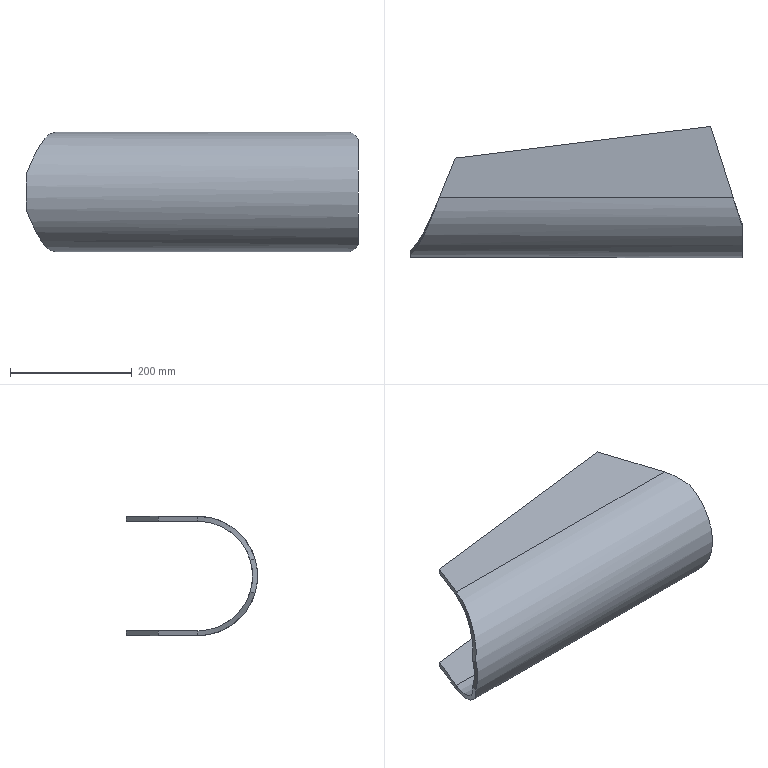Part | SolidWorks | features FlatPattern 1, SM3dBend 1, SMBaseFlange 1, SheetMetal 1 | 1 solid | 18 faces | box 545.7 x 215.495 x 196 mm | volume 1900724 mm3 | plane 12 | spline 4 | cylinder 2 | commonest cylinder face diameters 180 x1 196 x1
STEP:
#1=CARTESIAN_POINT('',(-26.166,147.655,180.));
#2=VERTEX_POINT('',#1);
#3=CARTESIAN_POINT('',(0.,213.,180.));
#4=VERTEX_POINT('',#3);
#5=CARTESIAN_POINT('',(-74.2,27.7,180.));
#6=DIRECTION('',(0.3717,0.9283,0.));
#7=VECTOR('',#6,1000.);
#8=LINE('',#5,#7);
#9=EDGE_CURVE('',#2,#4,#8,.T.);
#10=ORIENTED_EDGE('',*,*,#9,.F.);
#11=CARTESIAN_POINT('',(-26.166,147.655,188.));
#12=VERTEX_POINT('',#11);
#13=CARTESIAN_POINT('',(-26.166,147.655,180.));
#14=CARTESIAN_POINT('',(-26.166,147.655,182.667));
#15=CARTESIAN_POINT('',(-26.166,147.655,185.333));
#16=CARTESIAN_POINT('',(-26.166,147.655,188.));
#17=B_SPLINE_CURVE_WITH_KNOTS('',3,(#13,#14,#15,#16),.UNSPECIFIED.,.F.,.F.,(4,4),(0.,1.),.UNSPECIFIED.);
#18=EDGE_CURVE('',#2,#12,#17,.T.);
#19=ORIENTED_EDGE('',*,*,#18,.T.);
#20=CARTESIAN_POINT('',(0.,213.,188.));
#21=VERTEX_POINT('',#20);
#22=CARTESIAN_POINT('',(-74.2,27.7,188.));
#23=DIRECTION('',(0.3717,0.9283,0.));
#24=VECTOR('',#23,1000.);
#25=LINE('',#22,#24);
#26=EDGE_CURVE('',#12,#21,#25,.T.);
#27=ORIENTED_EDGE('',*,*,#26,.T.);
#28=CARTESIAN_POINT('',(0.,213.,188.));
#29=DIRECTION('',(0.,0.,-1.));
#30=VECTOR('',#29,1000.);
#31=LINE('',#28,#30);
#32=EDGE_CURVE('',#21,#4,#31,.T.);
#33=ORIENTED_EDGE('',*,*,#32,.T.);
#34=EDGE_LOOP('',(#10,#19,#27,#33));
#35=FACE_OUTER_BOUND('',#34,.T.);
#36=CARTESIAN_POINT('',(-74.2,27.7,188.));
#37=DIRECTION('',(-0.9283,0.3717,0.));
#38=DIRECTION('',(0.3717,0.9283,0.));
#39=AXIS2_PLACEMENT_3D('',#36,#37,#38);
#40=PLANE('',#39);
#41=ADVANCED_FACE('',(#35),#40,.T.);
#42=CARTESIAN_POINT('',(420.,265.15,188.));
#43=VERTEX_POINT('',#42);
#44=CARTESIAN_POINT('',(457.089,147.655,188.));
#45=VERTEX_POINT('',#44);
#46=CARTESIAN_POINT('',(420.,265.15,188.));
#47=DIRECTION('',(0.301,-0.9536,0.));
#48=VECTOR('',#47,1000.);
#49=LINE('',#46,#48);
#50=EDGE_CURVE('',#43,#45,#49,.T.);
#51=ORIENTED_EDGE('',*,*,#50,.T.);
#52=CARTESIAN_POINT('',(457.089,147.655,180.));
#53=VERTEX_POINT('',#52);
#54=CARTESIAN_POINT('',(457.089,147.655,188.));
#55=CARTESIAN_POINT('',(457.089,147.655,185.333));
#56=CARTESIAN_POINT('',(457.089,147.655,182.667));
#57=CARTESIAN_POINT('',(457.089,147.655,180.));
#58=B_SPLINE_CURVE_WITH_KNOTS('',3,(#54,#55,#56,#57),.UNSPECIFIED.,.F.,.F.,(4,4),(0.,1.),.UNSPECIFIED.);
#59=EDGE_CURVE('',#45,#53,#58,.T.);
#60=ORIENTED_EDGE('',*,*,#59,.T.);
#61=CARTESIAN_POINT('',(420.,265.15,180.));
#62=VERTEX_POINT('',#61);
#63=CARTESIAN_POINT('',(420.,265.15,180.));
#64=DIRECTION('',(0.301,-0.9536,0.));
#65=VECTOR('',#64,1000.);
#66=LINE('',#63,#65);
#67=EDGE_CURVE('',#62,#53,#66,.T.);
#68=ORIENTED_EDGE('',*,*,#67,.F.);
#69=CARTESIAN_POINT('',(420.,265.15,188.));
#70=DIRECTION('',(0.,0.,-1.));
#71=VECTOR('',#70,1000.);
#72=LINE('',#69,#71);
#73=EDGE_CURVE('',#43,#62,#72,.T.);
#74=ORIENTED_EDGE('',*,*,#73,.F.);
#75=EDGE_LOOP('',(#51,#60,#68,#74));
#76=FACE_OUTER_BOUND('',#75,.T.);
#77=CARTESIAN_POINT('',(420.,265.15,188.));
#78=DIRECTION('',(0.9536,0.301,0.));
#79=DIRECTION('',(0.301,-0.9536,0.));
#80=AXIS2_PLACEMENT_3D('',#77,#78,#79);
#81=PLANE('',#80);
#82=ADVANCED_FACE('',(#76),#81,.T.);
#83=ORIENTED_EDGE('',*,*,#67,.T.);
#84=CARTESIAN_POINT('',(-74.2,147.655,180.));
#85=DIRECTION('',(-1.,0.,0.));
#86=VECTOR('',#85,1000.);
#87=LINE('',#84,#86);
#88=EDGE_CURVE('',#53,#2,#87,.T.);
#89=ORIENTED_EDGE('',*,*,#88,.T.);
#90=ORIENTED_EDGE('',*,*,#9,.T.);
#91=CARTESIAN_POINT('',(0.,213.,180.));
#92=DIRECTION('',(0.9924,0.1232,0.));
#93=VECTOR('',#92,1000.);
#94=LINE('',#91,#93);
#95=EDGE_CURVE('',#4,#62,#94,.T.);
#96=ORIENTED_EDGE('',*,*,#95,.T.);
#97=EDGE_LOOP('',(#83,#89,#90,#96));
#98=FACE_OUTER_BOUND('',#97,.T.);
#99=CARTESIAN_POINT('',(-74.2,-203.787,180.));
#100=DIRECTION('',(0.,0.,-1.));
#101=DIRECTION('',(1.,0.,0.));
#102=AXIS2_PLACEMENT_3D('',#99,#100,#101);
#103=PLANE('',#102);
#104=ADVANCED_FACE('',(#98),#103,.T.);
#105=ORIENTED_EDGE('',*,*,#95,.F.);
#106=ORIENTED_EDGE('',*,*,#32,.F.);
#107=CARTESIAN_POINT('',(0.,213.,188.));
#108=DIRECTION('',(0.9924,0.1232,0.));
#109=VECTOR('',#108,1000.);
#110=LINE('',#107,#109);
#111=EDGE_CURVE('',#21,#43,#110,.T.);
#112=ORIENTED_EDGE('',*,*,#111,.T.);
#113=ORIENTED_EDGE('',*,*,#73,.T.);
#114=EDGE_LOOP('',(#105,#106,#112,#113));
#115=FACE_OUTER_BOUND('',#114,.T.);
#116=CARTESIAN_POINT('',(0.,213.,188.));
#117=DIRECTION('',(-0.1232,0.9924,0.));
#118=DIRECTION('',(0.9924,0.1232,0.));
#119=AXIS2_PLACEMENT_3D('',#116,#117,#118);
#120=PLANE('',#119);
#121=ADVANCED_FACE('',(#115),#120,.T.);
#122=CARTESIAN_POINT('',(-74.2,147.655,188.));
#123=DIRECTION('',(-1.,0.,0.));
#124=VECTOR('',#123,1000.);
#125=LINE('',#122,#124);
#126=EDGE_CURVE('',#45,#12,#125,.T.);
#127=ORIENTED_EDGE('',*,*,#126,.F.);
#128=ORIENTED_EDGE('',*,*,#50,.F.);
#129=ORIENTED_EDGE('',*,*,#111,.F.);
#130=ORIENTED_EDGE('',*,*,#26,.F.);
#131=EDGE_LOOP('',(#127,#128,#129,#130));
#132=FACE_OUTER_BOUND('',#131,.T.);
#133=CARTESIAN_POINT('',(-74.2,-203.787,188.));
#134=DIRECTION('',(0.,0.,-1.));
#135=DIRECTION('',(1.,0.,0.));
#136=AXIS2_PLACEMENT_3D('',#133,#134,#135);
#137=PLANE('',#136);
#138=ADVANCED_FACE('',(#132),#137,.F.);
#139=CARTESIAN_POINT('',(420.,265.15,0.));
#140=VERTEX_POINT('',#139);
#141=CARTESIAN_POINT('',(0.,213.,0.));
#142=VERTEX_POINT('',#141);
#143=CARTESIAN_POINT('',(420.,265.15,0.));
#144=DIRECTION('',(-0.9924,-0.1232,0.));
#145=VECTOR('',#144,1000.);
#146=LINE('',#143,#145);
#147=EDGE_CURVE('',#140,#142,#146,.T.);
#148=ORIENTED_EDGE('',*,*,#147,.F.);
#149=CARTESIAN_POINT('',(420.,265.15,-8.));
#150=VERTEX_POINT('',#149);
#151=CARTESIAN_POINT('',(420.,265.15,-8.));
#152=DIRECTION('',(0.,0.,1.));
#153=VECTOR('',#152,1000.);
#154=LINE('',#151,#153);
#155=EDGE_CURVE('',#150,#140,#154,.T.);
#156=ORIENTED_EDGE('',*,*,#155,.F.);
#157=CARTESIAN_POINT('',(0.,213.,-8.));
#158=VERTEX_POINT('',#157);
#159=CARTESIAN_POINT('',(420.,265.15,-8.));
#160=DIRECTION('',(-0.9924,-0.1232,0.));
#161=VECTOR('',#160,1000.);
#162=LINE('',#159,#161);
#163=EDGE_CURVE('',#150,#158,#162,.T.);
#164=ORIENTED_EDGE('',*,*,#163,.T.);
#165=CARTESIAN_POINT('',(0.,213.,-8.));
#166=DIRECTION('',(0.,0.,1.));
#167=VECTOR('',#166,1000.);
#168=LINE('',#165,#167);
#169=EDGE_CURVE('',#158,#142,#168,.T.);
#170=ORIENTED_EDGE('',*,*,#169,.T.);
#171=EDGE_LOOP('',(#148,#156,#164,#170));
#172=FACE_OUTER_BOUND('',#171,.T.);
#173=CARTESIAN_POINT('',(420.,265.15,-8.));
#174=DIRECTION('',(-0.1232,0.9924,0.));
#175=DIRECTION('',(-0.9924,-0.1232,0.));
#176=AXIS2_PLACEMENT_3D('',#173,#174,#175);
#177=PLANE('',#176);
#178=ADVANCED_FACE('',(#172),#177,.T.);
#179=CARTESIAN_POINT('',(457.089,147.655,-8.));
#180=VERTEX_POINT('',#179);
#181=CARTESIAN_POINT('',(471.5,102.,-8.));
#182=DIRECTION('',(-0.301,0.9536,0.));
#183=VECTOR('',#182,1000.);
#184=LINE('',#181,#183);
#185=EDGE_CURVE('',#180,#150,#184,.T.);
#186=ORIENTED_EDGE('',*,*,#185,.F.);
#187=CARTESIAN_POINT('',(-26.166,147.655,-8.));
#188=VERTEX_POINT('',#187);
#189=CARTESIAN_POINT('',(-74.2,147.655,-8.));
#190=DIRECTION('',(-1.,0.,0.));
#191=VECTOR('',#190,1000.);
#192=LINE('',#189,#191);
#193=EDGE_CURVE('',#180,#188,#192,.T.);
#194=ORIENTED_EDGE('',*,*,#193,.T.);
#195=CARTESIAN_POINT('',(0.,213.,-8.));
#196=DIRECTION('',(-0.3717,-0.9283,0.));
#197=VECTOR('',#196,1000.);
#198=LINE('',#195,#197);
#199=EDGE_CURVE('',#158,#188,#198,.T.);
#200=ORIENTED_EDGE('',*,*,#199,.F.);
#201=ORIENTED_EDGE('',*,*,#163,.F.);
#202=EDGE_LOOP('',(#186,#194,#200,#201));
#203=FACE_OUTER_BOUND('',#202,.T.);
#204=CARTESIAN_POINT('',(-74.2,203.787,-8.));
#205=DIRECTION('',(0.,0.,1.));
#206=DIRECTION('',(1.,0.,0.));
#207=AXIS2_PLACEMENT_3D('',#204,#205,#206);
#208=PLANE('',#207);
#209=ADVANCED_FACE('',(#203),#208,.F.);
#210=CARTESIAN_POINT('',(-26.166,147.655,0.));
#211=VERTEX_POINT('',#210);
#212=CARTESIAN_POINT('',(-26.166,147.655,0.));
#213=CARTESIAN_POINT('',(-26.166,147.655,-8.));
#214=B_SPLINE_CURVE_WITH_KNOTS('',1,(#212,#213),.UNSPECIFIED.,.F.,.F.,(2,2),(0.,1.),.UNSPECIFIED.);
#215=EDGE_CURVE('',#211,#188,#214,.T.);
#216=ORIENTED_EDGE('',*,*,#215,.F.);
#217=CARTESIAN_POINT('',(0.,213.,0.));
#218=DIRECTION('',(-0.3717,-0.9283,0.));
#219=VECTOR('',#218,1000.);
#220=LINE('',#217,#219);
#221=EDGE_CURVE('',#142,#211,#220,.T.);
#222=ORIENTED_EDGE('',*,*,#221,.F.);
#223=ORIENTED_EDGE('',*,*,#169,.F.);
#224=ORIENTED_EDGE('',*,*,#199,.T.);
#225=EDGE_LOOP('',(#216,#222,#223,#224));
#226=FACE_OUTER_BOUND('',#225,.T.);
#227=CARTESIAN_POINT('',(0.,213.,-8.));
#228=DIRECTION('',(-0.9283,0.3717,0.));
#229=DIRECTION('',(-0.3717,-0.9283,0.));
#230=AXIS2_PLACEMENT_3D('',#227,#228,#229);
#231=PLANE('',#230);
#232=ADVANCED_FACE('',(#226),#231,.T.);
#233=CARTESIAN_POINT('',(457.089,147.655,0.));
#234=VERTEX_POINT('',#233);
#235=CARTESIAN_POINT('',(-74.2,147.655,0.));
#236=DIRECTION('',(-1.,0.,0.));
#237=VECTOR('',#236,1000.);
#238=LINE('',#235,#237);
#239=EDGE_CURVE('',#234,#211,#238,.T.);
#240=ORIENTED_EDGE('',*,*,#239,.F.);
#241=CARTESIAN_POINT('',(471.5,102.,0.));
#242=DIRECTION('',(-0.301,0.9536,0.));
#243=VECTOR('',#242,1000.);
#244=LINE('',#241,#243);
#245=EDGE_CURVE('',#234,#140,#244,.T.);
#246=ORIENTED_EDGE('',*,*,#245,.T.);
#247=ORIENTED_EDGE('',*,*,#147,.T.);
#248=ORIENTED_EDGE('',*,*,#221,.T.);
#249=EDGE_LOOP('',(#240,#246,#247,#248));
#250=FACE_OUTER_BOUND('',#249,.T.);
#251=CARTESIAN_POINT('',(-74.2,203.787,0.));
#252=DIRECTION('',(0.,0.,1.));
#253=DIRECTION('',(1.,0.,0.));
#254=AXIS2_PLACEMENT_3D('',#251,#252,#253);
#255=PLANE('',#254);
#256=ADVANCED_FACE('',(#250),#255,.T.);
#257=CARTESIAN_POINT('',(457.089,147.655,-8.));
#258=CARTESIAN_POINT('',(457.089,147.655,0.));
#259=B_SPLINE_CURVE_WITH_KNOTS('',1,(#257,#258),.UNSPECIFIED.,.F.,.F.,(2,2),(0.,1.),.UNSPECIFIED.);
#260=EDGE_CURVE('',#180,#234,#259,.T.);
#261=ORIENTED_EDGE('',*,*,#260,.F.);
#262=ORIENTED_EDGE('',*,*,#185,.T.);
#263=ORIENTED_EDGE('',*,*,#155,.T.);
#264=ORIENTED_EDGE('',*,*,#245,.F.);
#265=EDGE_LOOP('',(#261,#262,#263,#264));
#266=FACE_OUTER_BOUND('',#265,.T.);
#267=CARTESIAN_POINT('',(471.5,102.,-8.));
#268=DIRECTION('',(0.9536,0.301,0.));
#269=DIRECTION('',(-0.301,0.9536,0.));
#270=AXIS2_PLACEMENT_3D('',#267,#268,#269);
#271=PLANE('',#270);
#272=ADVANCED_FACE('',(#266),#271,.T.);
#273=CARTESIAN_POINT('',(471.5,105.641,169.592));
#274=VERTEX_POINT('',#273);
#275=CARTESIAN_POINT('',(471.5,101.907,176.667));
#276=VERTEX_POINT('',#275);
#277=CARTESIAN_POINT('',(471.5,105.641,169.592));
#278=CARTESIAN_POINT('',(471.5,104.396,171.95));
#279=CARTESIAN_POINT('',(471.5,103.151,174.308));
#280=CARTESIAN_POINT('',(471.5,101.907,176.667));
#281=B_SPLINE_CURVE_WITH_KNOTS('',3,(#277,#278,#279,#280),.UNSPECIFIED.,.F.,.F.,(4,4),(0.,1.),.UNSPECIFIED.);
#282=EDGE_CURVE('',#274,#276,#281,.T.);
#283=ORIENTED_EDGE('',*,*,#282,.F.);
#284=CARTESIAN_POINT('',(471.5,105.641,169.592));
#285=CARTESIAN_POINT('',(469.098,112.084,172.993));
#286=CARTESIAN_POINT('',(466.696,118.941,175.607));
#287=CARTESIAN_POINT('',(461.892,133.085,179.111));
#288=CARTESIAN_POINT('',(459.491,140.369,180.));
#289=CARTESIAN_POINT('',(457.089,147.655,180.));
#290=B_SPLINE_CURVE_WITH_KNOTS('',3,(#284,#285,#286,#287,#288,#289),.UNSPECIFIED.,.F.,.F.,(4,2,4),(0.,0.5,1.),.UNSPECIFIED.);
#291=EDGE_CURVE('',#274,#53,#290,.T.);
#292=ORIENTED_EDGE('',*,*,#291,.T.);
#293=ORIENTED_EDGE('',*,*,#59,.F.);
#294=CARTESIAN_POINT('',(471.5,101.907,176.667));
#295=CARTESIAN_POINT('',(469.098,108.922,180.37));
#296=CARTESIAN_POINT('',(466.696,116.389,183.217));
#297=CARTESIAN_POINT('',(461.892,131.789,187.032));
#298=CARTESIAN_POINT('',(459.49,139.722,188.));
#299=CARTESIAN_POINT('',(457.089,147.655,188.));
#300=B_SPLINE_CURVE_WITH_KNOTS('',3,(#294,#295,#296,#297,#298,#299),.UNSPECIFIED.,.F.,.F.,(4,2,4),(0.,0.5,1.),.UNSPECIFIED.);
#301=EDGE_CURVE('',#276,#45,#300,.T.);
#302=ORIENTED_EDGE('',*,*,#301,.F.);
#303=EDGE_LOOP('',(#283,#292,#293,#302));
#304=FACE_OUTER_BOUND('',#303,.T.);
#305=CARTESIAN_POINT('',(471.5,101.907,176.667));
#306=CARTESIAN_POINT('',(469.098,108.922,180.37));
#307=CARTESIAN_POINT('',(466.696,116.389,183.217));
#308=CARTESIAN_POINT('',(461.892,131.789,187.032));
#309=CARTESIAN_POINT('',(459.491,139.722,188.));
#310=CARTESIAN_POINT('',(457.089,147.655,188.));
#311=CARTESIAN_POINT('',(471.5,105.641,169.592));
#312=CARTESIAN_POINT('',(469.098,112.084,172.993));
#313=CARTESIAN_POINT('',(466.696,118.941,175.607));
#314=CARTESIAN_POINT('',(461.892,133.085,179.111));
#315=CARTESIAN_POINT('',(459.491,140.369,180.));
#316=CARTESIAN_POINT('',(457.089,147.655,180.));
#317=B_SPLINE_SURFACE_WITH_KNOTS('',1,3,((#305,#306,#307,#308,#309,#310),(#311,#312,#313,#314,#315,#316)),.UNSPECIFIED.,.F.,.F.,.F.,(2,2),(4,2,4),(0.,1.),(0.,0.5,1.),.UNSPECIFIED.);
#318=ADVANCED_FACE('',(#304),#317,.T.);
#319=ORIENTED_EDGE('',*,*,#18,.F.);
#320=CARTESIAN_POINT('',(-74.2,61.534,116.139));
#321=VERTEX_POINT('',#320);
#322=CARTESIAN_POINT('',(-26.166,147.655,180.));
#323=CARTESIAN_POINT('',(-30.169,138.083,180.));
#324=CARTESIAN_POINT('',(-34.172,128.515,178.46));
#325=CARTESIAN_POINT('',(-42.178,110.339,172.457));
#326=CARTESIAN_POINT('',(-46.18,101.735,167.994));
#327=CARTESIAN_POINT('',(-54.186,86.36,156.592));
#328=CARTESIAN_POINT('',(-58.189,79.59,149.656));
#329=CARTESIAN_POINT('',(-66.194,68.566,134.007));
#330=CARTESIAN_POINT('',(-70.197,64.314,125.298));
#331=CARTESIAN_POINT('',(-74.2,61.534,116.139));
#332=B_SPLINE_CURVE_WITH_KNOTS('',3,(#322,#323,#324,#325,#326,#327,#328,#329,#330,#331),.UNSPECIFIED.,.F.,.F.,(4,2,2,2,4),(0.,0.25,0.5,0.75,1.),.UNSPECIFIED.);
#333=EDGE_CURVE('',#2,#321,#332,.T.);
#334=ORIENTED_EDGE('',*,*,#333,.T.);
#335=CARTESIAN_POINT('',(-74.2,53.879,118.463));
#336=VERTEX_POINT('',#335);
#337=CARTESIAN_POINT('',(-74.2,61.534,116.139));
#338=CARTESIAN_POINT('',(-74.2,53.879,118.463));
#339=B_SPLINE_CURVE_WITH_KNOTS('',1,(#337,#338),.UNSPECIFIED.,.F.,.F.,(2,2),(0.,1.),.UNSPECIFIED.);
#340=EDGE_CURVE('',#321,#336,#339,.T.);
#341=ORIENTED_EDGE('',*,*,#340,.T.);
#342=CARTESIAN_POINT('',(-26.166,147.655,188.));
#343=CARTESIAN_POINT('',(-28.168,142.444,188.));
#344=CARTESIAN_POINT('',(-30.169,137.233,187.584));
#345=CARTESIAN_POINT('',(-34.172,126.944,185.928));
#346=CARTESIAN_POINT('',(-36.173,121.866,184.689));
#347=CARTESIAN_POINT('',(-40.176,111.97,181.421));
#348=CARTESIAN_POINT('',(-42.178,107.153,179.391));
#349=CARTESIAN_POINT('',(-46.18,97.902,174.592));
#350=CARTESIAN_POINT('',(-48.182,93.468,171.823));
#351=CARTESIAN_POINT('',(-52.185,85.097,165.615));
#352=CARTESIAN_POINT('',(-54.186,81.159,162.177));
#353=CARTESIAN_POINT('',(-58.189,73.88,154.719));
#354=CARTESIAN_POINT('',(-60.19,70.539,150.699));
#355=CARTESIAN_POINT('',(-64.193,64.537,142.179));
#356=CARTESIAN_POINT('',(-66.194,61.877,137.679));
#357=CARTESIAN_POINT('',(-70.197,57.304,128.314));
#358=CARTESIAN_POINT('',(-72.199,55.393,123.449));
#359=CARTESIAN_POINT('',(-74.2,53.879,118.463));
#360=B_SPLINE_CURVE_WITH_KNOTS('',3,(#342,#343,#344,#345,#346,#347,#348,#349,#350,#351,#352,#353,#354,#355,#356,#357,#358,#359),.UNSPECIFIED.,.F.,.F.,(4,2,2,2,2,2,2,2,4),(0.,0.125,0.25,0.375,0.5,0.625,0.75,0.875,1.),.UNSPECIFIED.);
#361=EDGE_CURVE('',#12,#336,#360,.T.);
#362=ORIENTED_EDGE('',*,*,#361,.F.);
#363=EDGE_LOOP('',(#319,#334,#341,#362));
#364=FACE_OUTER_BOUND('',#363,.T.);
#365=CARTESIAN_POINT('',(-26.166,147.655,188.));
#366=CARTESIAN_POINT('',(-30.169,137.233,188.));
#367=CARTESIAN_POINT('',(-34.172,126.813,186.324));
#368=CARTESIAN_POINT('',(-42.178,107.022,179.786));
#369=CARTESIAN_POINT('',(-46.18,97.654,174.926));
#370=CARTESIAN_POINT('',(-54.186,80.911,162.511));
#371=CARTESIAN_POINT('',(-58.189,73.54,154.958));
#372=CARTESIAN_POINT('',(-66.194,61.536,137.919));
#373=CARTESIAN_POINT('',(-70.197,56.906,128.436));
#374=CARTESIAN_POINT('',(-74.2,53.879,118.463));
#375=CARTESIAN_POINT('',(-26.166,147.655,180.));
#376=CARTESIAN_POINT('',(-30.169,138.083,180.));
#377=CARTESIAN_POINT('',(-34.172,128.515,178.46));
#378=CARTESIAN_POINT('',(-42.178,110.339,172.457));
#379=CARTESIAN_POINT('',(-46.18,101.735,167.994));
#380=CARTESIAN_POINT('',(-54.186,86.36,156.592));
#381=CARTESIAN_POINT('',(-58.189,79.59,149.656));
#382=CARTESIAN_POINT('',(-66.194,68.566,134.007));
#383=CARTESIAN_POINT('',(-70.197,64.314,125.298));
#384=CARTESIAN_POINT('',(-74.2,61.534,116.139));
#385=B_SPLINE_SURFACE_WITH_KNOTS('',1,3,((#365,#366,#367,#368,#369,#370,#371,#372,#373,#374),(#375,#376,#377,#378,#379,#380,#381,#382,#383,#384)),.UNSPECIFIED.,.F.,.F.,.F.,(2,2),(4,2,2,2,4),(0.,1.),(0.,0.25,0.5,0.75,1.),.UNSPECIFIED.);
#386=ADVANCED_FACE('',(#364),#385,.T.);
#387=ORIENTED_EDGE('',*,*,#340,.F.);
#388=CARTESIAN_POINT('',(-74.2,61.534,63.861));
#389=VERTEX_POINT('',#388);
#390=CARTESIAN_POINT('',(-74.2,147.655,90.));
#391=DIRECTION('',(1.,0.,0.));
#392=DIRECTION('',(0.,0.,1.));
#393=AXIS2_PLACEMENT_3D('',#390,#391,#392);
#394=CIRCLE('',#393,90.);
#395=EDGE_CURVE('',#321,#389,#394,.T.);
#396=ORIENTED_EDGE('',*,*,#395,.T.);
#397=CARTESIAN_POINT('',(-74.2,53.879,61.537));
#398=VERTEX_POINT('',#397);
#399=CARTESIAN_POINT('',(-74.2,61.534,63.861));
#400=CARTESIAN_POINT('',(-74.2,58.983,63.086));
#401=CARTESIAN_POINT('',(-74.2,56.431,62.312));
#402=CARTESIAN_POINT('',(-74.2,53.879,61.537));
#403=B_SPLINE_CURVE_WITH_KNOTS('',3,(#399,#400,#401,#402),.UNSPECIFIED.,.F.,.F.,(4,4),(0.,1.),.UNSPECIFIED.);
#404=EDGE_CURVE('',#389,#398,#403,.T.);
#405=ORIENTED_EDGE('',*,*,#404,.T.);
#406=CARTESIAN_POINT('',(-74.2,147.655,90.));
#407=DIRECTION('',(1.,0.,0.));
#408=DIRECTION('',(0.,0.,1.));
#409=AXIS2_PLACEMENT_3D('',#406,#407,#408);
#410=CIRCLE('',#409,98.);
#411=EDGE_CURVE('',#336,#398,#410,.T.);
#412=ORIENTED_EDGE('',*,*,#411,.F.);
#413=EDGE_LOOP('',(#387,#396,#405,#412));
#414=FACE_OUTER_BOUND('',#413,.T.);
#415=CARTESIAN_POINT('',(-74.2,147.655,90.));
#416=DIRECTION('',(-1.,0.,0.));
#417=DIRECTION('',(0.,0.,1.));
#418=AXIS2_PLACEMENT_3D('',#415,#416,#417);
#419=PLANE('',#418);
#420=ADVANCED_FACE('',(#414),#419,.T.);
#421=ORIENTED_EDGE('',*,*,#404,.F.);
#422=CARTESIAN_POINT('',(-74.2,61.534,63.861));
#423=CARTESIAN_POINT('',(-70.197,64.314,54.702));
#424=CARTESIAN_POINT('',(-66.194,68.566,45.993));
#425=CARTESIAN_POINT('',(-58.189,79.59,30.344));
#426=CARTESIAN_POINT('',(-54.186,86.36,23.408));
#427=CARTESIAN_POINT('',(-46.18,101.735,12.006));
#428=CARTESIAN_POINT('',(-42.178,110.339,7.543));
#429=CARTESIAN_POINT('',(-34.172,128.515,1.54));
#430=CARTESIAN_POINT('',(-30.169,138.083,0.));
#431=CARTESIAN_POINT('',(-26.166,147.655,0.));
#432=B_SPLINE_CURVE_WITH_KNOTS('',3,(#422,#423,#424,#425,#426,#427,#428,#429,#430,#431),.UNSPECIFIED.,.F.,.F.,(4,2,2,2,4),(0.,0.25,0.5,0.75,1.),.UNSPECIFIED.);
#433=EDGE_CURVE('',#389,#211,#432,.T.);
#434=ORIENTED_EDGE('',*,*,#433,.T.);
#435=ORIENTED_EDGE('',*,*,#215,.T.);
#436=CARTESIAN_POINT('',(-74.2,53.879,61.537));
#437=CARTESIAN_POINT('',(-72.199,55.393,56.551));
#438=CARTESIAN_POINT('',(-70.197,57.304,51.686));
#439=CARTESIAN_POINT('',(-66.194,61.877,42.321));
#440=CARTESIAN_POINT('',(-64.193,64.537,37.821));
#441=CARTESIAN_POINT('',(-60.19,70.539,29.301));
#442=CARTESIAN_POINT('',(-58.189,73.88,25.281));
#443=CARTESIAN_POINT('',(-54.186,81.159,17.823));
#444=CARTESIAN_POINT('',(-52.185,85.097,14.385));
#445=CARTESIAN_POINT('',(-48.182,93.468,8.177));
#446=CARTESIAN_POINT('',(-46.18,97.902,5.408));
#447=CARTESIAN_POINT('',(-42.178,107.153,0.6092));
#448=CARTESIAN_POINT('',(-40.176,111.97,-1.421));
#449=CARTESIAN_POINT('',(-36.173,121.866,-4.689));
#450=CARTESIAN_POINT('',(-34.172,126.944,-5.928));
#451=CARTESIAN_POINT('',(-30.169,137.233,-7.584));
#452=CARTESIAN_POINT('',(-28.168,142.444,-8.));
#453=CARTESIAN_POINT('',(-26.166,147.655,-8.));
#454=B_SPLINE_CURVE_WITH_KNOTS('',3,(#436,#437,#438,#439,#440,#441,#442,#443,#444,#445,#446,#447,#448,#449,#450,#451,#452,#453),.UNSPECIFIED.,.F.,.F.,(4,2,2,2,2,2,2,2,4),(0.,0.125,0.25,0.375,0.5,0.625,0.75,0.875,1.),.UNSPECIFIED.);
#455=EDGE_CURVE('',#398,#188,#454,.T.);
#456=ORIENTED_EDGE('',*,*,#455,.F.);
#457=EDGE_LOOP('',(#421,#434,#435,#456));
#458=FACE_OUTER_BOUND('',#457,.T.);
#459=CARTESIAN_POINT('',(-74.2,53.879,61.537));
#460=CARTESIAN_POINT('',(-70.197,56.906,51.564));
#461=CARTESIAN_POINT('',(-66.194,61.536,42.081));
#462=CARTESIAN_POINT('',(-58.189,73.54,25.042));
#463=CARTESIAN_POINT('',(-54.186,80.911,17.489));
#464=CARTESIAN_POINT('',(-46.18,97.654,5.074));
#465=CARTESIAN_POINT('',(-42.178,107.022,0.2137));
#466=CARTESIAN_POINT('',(-34.172,126.813,-6.324));
#467=CARTESIAN_POINT('',(-30.169,137.233,-8.));
#468=CARTESIAN_POINT('',(-26.166,147.655,-8.));
#469=CARTESIAN_POINT('',(-74.2,61.534,63.861));
#470=CARTESIAN_POINT('',(-70.197,64.314,54.702));
#471=CARTESIAN_POINT('',(-66.194,68.566,45.993));
#472=CARTESIAN_POINT('',(-58.189,79.59,30.344));
#473=CARTESIAN_POINT('',(-54.186,86.36,23.408));
#474=CARTESIAN_POINT('',(-46.18,101.735,12.006));
#475=CARTESIAN_POINT('',(-42.178,110.339,7.543));
#476=CARTESIAN_POINT('',(-34.172,128.515,1.54));
#477=CARTESIAN_POINT('',(-30.169,138.083,0.));
#478=CARTESIAN_POINT('',(-26.166,147.655,0.));
#479=B_SPLINE_SURFACE_WITH_KNOTS('',1,3,((#459,#460,#461,#462,#463,#464,#465,#466,#467,#468),(#469,#470,#471,#472,#473,#474,#475,#476,#477,#478)),.UNSPECIFIED.,.F.,.F.,.F.,(2,2),(4,2,2,2,4),(0.,1.),(0.,0.25,0.5,0.75,1.),.UNSPECIFIED.);
#480=ADVANCED_FACE('',(#458),#479,.T.);
#481=ORIENTED_EDGE('',*,*,#260,.T.);
#482=CARTESIAN_POINT('',(471.5,105.641,10.408));
#483=VERTEX_POINT('',#482);
#484=CARTESIAN_POINT('',(457.089,147.655,0.));
#485=CARTESIAN_POINT('',(459.491,140.369,0.));
#486=CARTESIAN_POINT('',(461.892,133.085,0.8889));
#487=CARTESIAN_POINT('',(466.696,118.941,4.393));
#488=CARTESIAN_POINT('',(469.098,112.084,7.007));
#489=CARTESIAN_POINT('',(471.5,105.641,10.408));
#490=B_SPLINE_CURVE_WITH_KNOTS('',3,(#484,#485,#486,#487,#488,#489),.UNSPECIFIED.,.F.,.F.,(4,2,4),(0.,0.5,1.),.UNSPECIFIED.);
#491=EDGE_CURVE('',#234,#483,#490,.T.);
#492=ORIENTED_EDGE('',*,*,#491,.T.);
#493=CARTESIAN_POINT('',(471.5,101.907,3.333));
#494=VERTEX_POINT('',#493);
#495=CARTESIAN_POINT('',(471.5,105.641,10.408));
#496=CARTESIAN_POINT('',(471.5,101.907,3.333));
#497=B_SPLINE_CURVE_WITH_KNOTS('',1,(#495,#496),.UNSPECIFIED.,.F.,.F.,(2,2),(0.,1.),.UNSPECIFIED.);
#498=EDGE_CURVE('',#483,#494,#497,.T.);
#499=ORIENTED_EDGE('',*,*,#498,.T.);
#500=CARTESIAN_POINT('',(457.089,147.655,-8.));
#501=CARTESIAN_POINT('',(459.49,139.722,-8.));
#502=CARTESIAN_POINT('',(461.892,131.789,-7.032));
#503=CARTESIAN_POINT('',(466.696,116.389,-3.217));
#504=CARTESIAN_POINT('',(469.098,108.922,-0.3698));
#505=CARTESIAN_POINT('',(471.5,101.907,3.333));
#506=B_SPLINE_CURVE_WITH_KNOTS('',3,(#500,#501,#502,#503,#504,#505),.UNSPECIFIED.,.F.,.F.,(4,2,4),(0.,0.5,1.),.UNSPECIFIED.);
#507=EDGE_CURVE('',#180,#494,#506,.T.);
#508=ORIENTED_EDGE('',*,*,#507,.F.);
#509=EDGE_LOOP('',(#481,#492,#499,#508));
#510=FACE_OUTER_BOUND('',#509,.T.);
#511=CARTESIAN_POINT('',(457.089,147.655,-8.));
#512=CARTESIAN_POINT('',(459.491,139.722,-8.));
#513=CARTESIAN_POINT('',(461.892,131.789,-7.032));
#514=CARTESIAN_POINT('',(466.696,116.389,-3.217));
#515=CARTESIAN_POINT('',(469.098,108.922,-0.3699));
#516=CARTESIAN_POINT('',(471.5,101.907,3.333));
#517=CARTESIAN_POINT('',(457.089,147.655,0.));
#518=CARTESIAN_POINT('',(459.491,140.369,0.));
#519=CARTESIAN_POINT('',(461.892,133.085,0.8889));
#520=CARTESIAN_POINT('',(466.696,118.941,4.393));
#521=CARTESIAN_POINT('',(469.098,112.084,7.007));
#522=CARTESIAN_POINT('',(471.5,105.641,10.408));
#523=B_SPLINE_SURFACE_WITH_KNOTS('',1,3,((#511,#512,#513,#514,#515,#516),(#517,#518,#519,#520,#521,#522)),.UNSPECIFIED.,.F.,.F.,.F.,(2,2),(4,2,4),(0.,1.),(0.,0.5,1.),.UNSPECIFIED.);
#524=ADVANCED_FACE('',(#510),#523,.T.);
#525=ORIENTED_EDGE('',*,*,#507,.T.);
#526=CARTESIAN_POINT('',(471.5,147.655,90.));
#527=DIRECTION('',(-1.,0.,0.));
#528=DIRECTION('',(0.,0.,-1.));
#529=AXIS2_PLACEMENT_3D('',#526,#527,#528);
#530=CIRCLE('',#529,98.);
#531=EDGE_CURVE('',#494,#276,#530,.T.);
#532=ORIENTED_EDGE('',*,*,#531,.T.);
#533=ORIENTED_EDGE('',*,*,#301,.T.);
#534=ORIENTED_EDGE('',*,*,#126,.T.);
#535=ORIENTED_EDGE('',*,*,#361,.T.);
#536=ORIENTED_EDGE('',*,*,#411,.T.);
#537=ORIENTED_EDGE('',*,*,#455,.T.);
#538=ORIENTED_EDGE('',*,*,#193,.F.);
#539=EDGE_LOOP('',(#525,#532,#533,#534,#535,#536,#537,#538));
#540=FACE_OUTER_BOUND('',#539,.T.);
#541=CARTESIAN_POINT('',(835.993,147.655,90.));
#542=DIRECTION('',(-1.,0.,0.));
#543=DIRECTION('',(0.,0.,1.));
#544=AXIS2_PLACEMENT_3D('',#541,#542,#543);
#545=CYLINDRICAL_SURFACE('',#544,98.);
#546=ADVANCED_FACE('',(#540),#545,.T.);
#547=CARTESIAN_POINT('',(471.5,147.655,90.));
#548=DIRECTION('',(-1.,0.,0.));
#549=DIRECTION('',(0.,0.,1.));
#550=AXIS2_PLACEMENT_3D('',#547,#548,#549);
#551=CIRCLE('',#550,90.);
#552=EDGE_CURVE('',#483,#274,#551,.T.);
#553=ORIENTED_EDGE('',*,*,#552,.T.);
#554=ORIENTED_EDGE('',*,*,#282,.T.);
#555=ORIENTED_EDGE('',*,*,#531,.F.);
#556=ORIENTED_EDGE('',*,*,#498,.F.);
#557=EDGE_LOOP('',(#553,#554,#555,#556));
#558=FACE_OUTER_BOUND('',#557,.T.);
#559=CARTESIAN_POINT('',(471.5,147.655,90.));
#560=DIRECTION('',(1.,0.,0.));
#561=DIRECTION('',(0.,0.,-1.));
#562=AXIS2_PLACEMENT_3D('',#559,#560,#561);
#563=PLANE('',#562);
#564=ADVANCED_FACE('',(#558),#563,.T.);
#565=ORIENTED_EDGE('',*,*,#491,.F.);
#566=ORIENTED_EDGE('',*,*,#239,.T.);
#567=ORIENTED_EDGE('',*,*,#433,.F.);
#568=ORIENTED_EDGE('',*,*,#395,.F.);
#569=ORIENTED_EDGE('',*,*,#333,.F.);
#570=ORIENTED_EDGE('',*,*,#88,.F.);
#571=ORIENTED_EDGE('',*,*,#291,.F.);
#572=ORIENTED_EDGE('',*,*,#552,.F.);
#573=EDGE_LOOP('',(#565,#566,#567,#568,#569,#570,#571,#572));
#574=FACE_OUTER_BOUND('',#573,.T.);
#575=CARTESIAN_POINT('',(835.993,147.655,90.));
#576=DIRECTION('',(-1.,0.,0.));
#577=DIRECTION('',(0.,0.,1.));
#578=AXIS2_PLACEMENT_3D('',#575,#576,#577);
#579=CYLINDRICAL_SURFACE('',#578,90.);
#580=ADVANCED_FACE('',(#574),#579,.F.);
#581=CLOSED_SHELL('',(#41,#82,#104,#121,#138,#178,#209,#232,#256,#272,#318,#386,#420,#480,#524,#546,#564,#580));
#582=MANIFOLD_SOLID_BREP('',#581);
#583=CARTESIAN_POINT('',(0.,0.,0.));
#584=DIRECTION('',(0.,0.,1.));
#585=DIRECTION('',(1.,0.,0.));
#586=AXIS2_PLACEMENT_3D('',#583,#584,#585);
#587=(LENGTH_UNIT()NAMED_UNIT(*)SI_UNIT(.MILLI.,.METRE.));
#588=UNCERTAINTY_MEASURE_WITH_UNIT(LENGTH_MEASURE(0.00001),#587,'','');
#589=(NAMED_UNIT(*)PLANE_ANGLE_UNIT()SI_UNIT($,.RADIAN.));
#590=(NAMED_UNIT(*)SI_UNIT($,.STERADIAN.)SOLID_ANGLE_UNIT());
#591=(GEOMETRIC_REPRESENTATION_CONTEXT(3)GLOBAL_UNCERTAINTY_ASSIGNED_CONTEXT((#588))GLOBAL_UNIT_ASSIGNED_CONTEXT((#587,#589,#590))REPRESENTATION_CONTEXT('',''));
#592=ADVANCED_BREP_SHAPE_REPRESENTATION('',(#582,#586),#591);